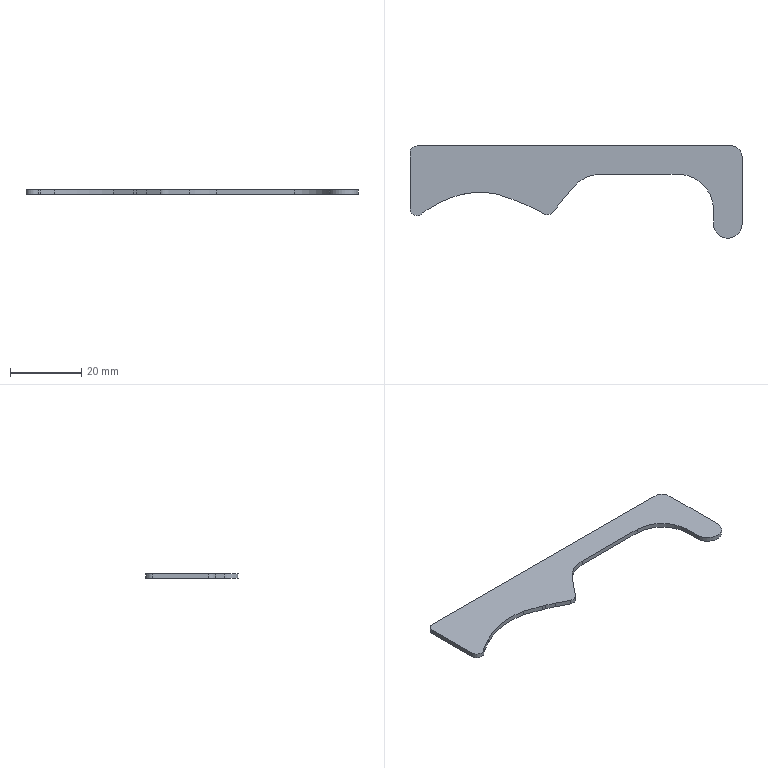Part | STEP file | gslz 2016.10.28-13_id202_x_t | 1 solid | 22 faces | box 93.419 x 26 x 1.25 mm | volume 1583 mm3 | plane 13 | cylinder 9 | commonest cylinder face diameters 4 x4 20 x2 6 x1 8 x1 46.953 x1